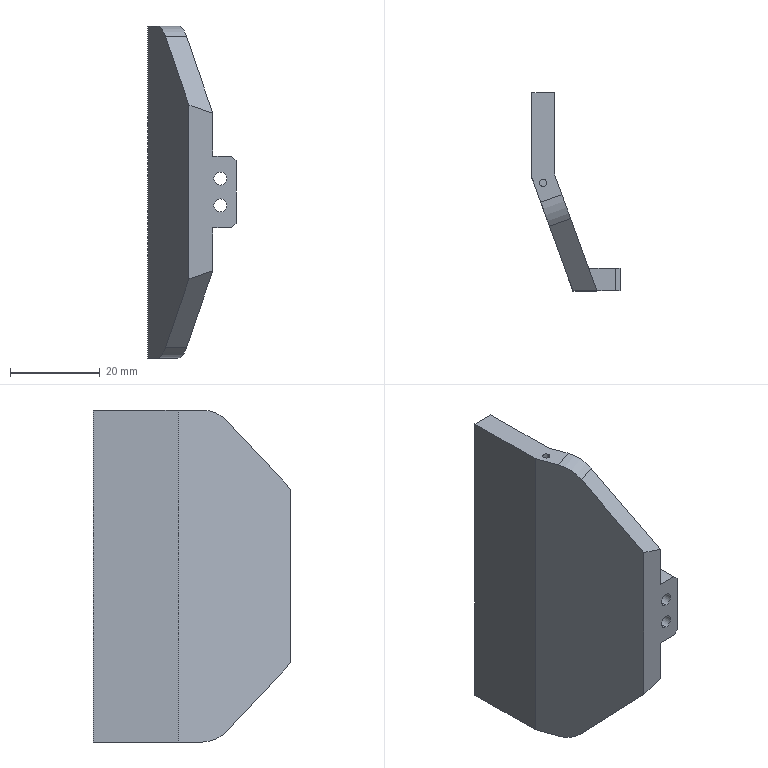NC program | NX | posted with a generic post | part box 19.643 x 44.061 x 74 mm
Lines 1 to 826 of 2613:
N10 G17 G21 G94 G90
(ADAPTIVE_MILLING , TOOL : D8开粗)
N12 T02 M6
N14 G54
N16 G17 G0 G90 X-47.558 Y-38.993 B0. C0. S6500 M3
N18 G43 Z30. H2
N20 Z-6.403
N22 G94 G1 X-47.492 Y-39.128 Z-7.34 F2500.
N24 X-47.426 Y-39.263 Z-7.711
N26 X-47.36 Y-39.398 Z-7.983
N28 X-47.294 Y-39.533 Z-8.203
N30 X-47.228 Y-39.667 Z-8.387
N32 X-47.163 Y-39.802 Z-8.546
N34 X-47.097 Y-39.937 Z-8.683
N36 X-47.031 Y-40.072 Z-8.803
N38 X-46.965 Y-40.207 Z-8.909
N40 X-46.899 Y-40.341 Z-9.001
N42 X-46.834 Y-40.476 Z-9.082
N44 X-46.768 Y-40.611 Z-9.153
N46 X-46.702 Y-40.746 Z-9.213
N48 X-46.636 Y-40.881 Z-9.265
N50 X-46.57 Y-41.015 Z-9.308
N52 X-46.505 Y-41.15 Z-9.343
N54 X-46.439 Y-41.285 Z-9.369
N56 X-46.373 Y-41.42 Z-9.388
N58 X-46.307 Y-41.554 Z-9.399
N60 X-46.241 Y-41.689 Z-9.403
N62 X-45.513 Y-43.182
N64 G3 X-43.999 Y-43.007 R0.808
N66 X-43.585 Y-39.981 R11.665
N68 X-43.499 Y-30.169 R281.498
N70 G1 X-43.498 Y-0.807
N72 G2 X-41.632 Y2.597 R4.521
N74 X-37.843 Y4.119 R8.422
N76 X-32.61 Y4.472 R35.063
N78 G1 X-24.735 Y4.499
N80 X38.215 Y4.497
N82 G2 X41.601 Y2.603 R4.555
N84 X43.114 Y-1.166 R8.498
N86 X43.471 Y-6.398 R34.669
N88 G1 X43.498 Y-14.273
N90 X43.499 Y-42.121
N92 G3 X43.654 Y-43.509 R4.062
N94 G1 X43.805 Y-43.722
N96 G3 X45.057 Y-43.547 R0.8
N98 X45.149 Y-42.984 Z-9.366 R0.86
N100 G1 X45.038 Y-41.99 Z-9.303
N102 G2 X46.322 Y-41.205 R0.804 F15000.
N104 G1 X46.546 Y-41.378
N106 X46.759 Y-41.564
N108 G2 X46.943 Y-41.919 R0.832
N110 X46.411 Y-42.865 Z-9.378 R0.816 F2500.
N112 G1 X46.05 Y-43.022 Z-9.403
N114 X44.62 Y-43.645
N116 G2 X43.577 Y-43.252 R0.8
N118 X43.283 Y-41.381 R6.234
N120 X43.199 Y-34.743 R157.881
N122 G1 X43.197 Y-11.856
N124 G3 X43.067 Y-3.796 R144.834
N126 X42.299 Y0.279 R13.658
N128 X39.053 Y3.396 R5.427
N130 X35.047 Y4.114 R12.873
N132 X26.723 Y4.198 R203.788
N134 G1 X-27.902 Y4.197
N136 G3 X-35.437 Y4.053 R122.134
N138 X-39.461 Y3.235 R12.737
N140 X-42.391 Y0.085 R5.405
N142 X-43.114 Y-3.92 R12.823
N144 X-43.199 Y-12.244 R201.638
N146 G1 Y-32.018
N148 G2 X-43.322 Y-40.262 R153.123
N150 X-43.694 Y-43.231 R28.567
N152 G1 X-43.797 Y-43.431
N154 G2 X-45.117 Y-43.393 R0.8
N156 G1 X-45.352 Y-43.028
N158 X-46.207 Y-41.697 Z-9.303
N160 G2 X-46.314 Y-40.913 R0.813 F15000.
N162 G1 X-46.22 Y-40.669
N164 X-46.111 Y-40.432
N166 G2 X-44.671 Y-41.106 R0.8
N168 G1 X-44.889 Y-41.749
N170 X-45.149 Y-42.535 Z-9.356 F2500.
N172 G3 X-44.987 Y-43.242 Z-9.403 R0.799
N174 X-43.655 Y-43.072 R0.8
N176 X-42.97 Y-40.45 R7.766
N178 X-42.712 Y-33.973 R62.177
N180 G1 X-42.699 Y-27.244
N182 X-42.698 Y-10.544
N184 G2 X-42.568 Y-3.91 R96.862
N186 X-41.825 Y-0.636 R9.476
N188 X-38.335 Y2.524 R6.635
N190 X-33.772 Y3.511 R14.696
N192 X-26.688 Y3.693 R98.536
N194 G1 X-21.252 Y3.713
N196 G3 X-20.829 Y3.886 R5.378
N198 G2 X-19.332 Y4.15 R4.834
N200 G1 X19.368
N202 G2 X21.088 Y3.911 R18.579
N204 G3 X26.996 Y3.706 R60.488
N206 G2 X34.526 Y3.606 R169.703
N208 X38.051 Y2.955 R11.35
N210 X41.428 Y-0.465 R6.487
N212 X42.494 Y-5.048 R13.967
N214 X42.694 Y-12.693 R97.602
N216 G1 X42.698 Y-17.156
N218 X42.7 Y-35.24
N220 G3 X42.822 Y-41.261 R87.83
N222 X43.278 Y-43.288 R5.747
N224 X43.917 Y-43.94 R1.116
N226 X44.864 Y-43.48 R0.8
N228 G1 X45.366 Y-41.98 Z-9.303
N230 X45.656 Y-41.11 F15000.
N232 X45.685 Y-40.985
N234 X45.697 Y-40.857
N236 Y-13.166
N238 G3 X45.047 Y-5.309 R47.833
N240 G1 X44.798 Y-3.797
N242 X44.532 Y-2.289
N244 G3 X43.545 Y0.807 R17.168
N246 X42.04 Y3.094 R7.735
N248 X40.398 Y4.429 R11.341
N250 X38.041 Y5.448 R8.159
N252 X35.622 Y5.838 R12.101
N254 G1 X22.704 Y6.583
N256 G3 X22.346 Y6.521 R0.848
N258 G1 X20.925 Y5.92
N260 X20.479 Y5.733 Z-9.334 F2500.
N262 X20.038 Y5.538 Z-9.364
N264 G3 X19.649 Y5.08 Z-9.403 R0.8
N266 X20.187 Y4.065 R0.8
N268 X22.184 Y3.527 R16.655
N270 X27.364 Y3.224 R38.873
N272 G2 X34.129 Y3.086 R136.962
N274 X37.786 Y2.097 R8.143
N276 X41.056 Y-1.974 R7.812
N278 X42.026 Y-7.039 R17.772
N280 X42.194 Y-14.911 R127.356
N282 G1 X42.198 Y-19.486
N284 X42.2 Y-34.378
N286 G3 X42.324 Y-40.628 R91.007
N288 X42.958 Y-43.254 R6.736
N290 X43.796 Y-43.971 R1.278
N292 G1 X43.871 Y-43.98
N294 G3 X44.579 Y-43.613 R0.801
N296 G1 X44.778 Y-43.303
N298 X45.632 Y-41.971 Z-9.303
N300 G2 X45.899 Y-41.635 R1.18 F15000.
N302 X46.388 Y-41.463 R0.808
N304 X46.821 Y-41.5 R1.214
N306 X47.296 Y-41.918 R0.804
N308 X46.786 Y-43.034 Z-9.391 R0.808 F2500.
N310 G1 X46.61 Y-43.098 Z-9.403
N312 X44.303 Y-43.931
N314 G2 X43.053 Y-43.523 R1.08
N316 X42.215 Y-41.341 R4.767
N318 X41.924 Y-36.863 R30.864
N320 G1 X41.898 Y-29.455
N322 X41.896 Y-16.293
N324 G3 X41.725 Y-7.371 R143.397
N326 X40.788 Y-2.452 R17.424
N328 X35.35 Y2.37 R7.418
N330 X30.735 Y2.861 R22.027
N332 G2 X24.11 Y3.051 R164.675
N334 X21.769 Y3.397 R10.417
N336 G1 X21.67 Y3.451
N338 G2 X21.32 Y4.104 R0.802
N340 X21.44 Y4.561 Z-9.373 R1.113
N342 G1 X21.858 Y5.584 Z-9.303
N344 X22.228 Y6.486 F15000.
N346 G2 X22.685 Y6.939 R0.865
N348 X23.09 Y5.434 R-0.8
N350 G1 X22.248 Y5.404
N352 X21.687 Y5.388 Z-9.339 F2500.
N354 X21.126 Y5.356 Z-9.374
N356 G3 X20.722 Y5.153 Z-9.403 R0.833
N358 X20.905 Y3.856 R0.8
N360 G2 X21.96 Y3.258 R7.341
N362 G3 X24.63 Y2.64 R8.31
N364 X30.643 Y2.357 R99.943
N366 G2 X34.91 Y1.801 R18.389
N368 X39.949 Y-2.699 R7.827
N370 X41.131 Y-7.641 R15.896
N372 X41.387 Y-14.984 R82.682
N374 G1 X41.398 Y-22.001
N376 G3 X41.449 Y-37.436 R879.459
N378 X41.892 Y-41.698 R20.187
N380 X42.926 Y-43.702 R4.096
N382 X43.88 Y-43.982 R1.117
N384 G2 X42.623 Y-43.495 R1.307
N386 X41.579 Y-41.16 R5.176
N388 X41.15 Y-36.518 R25.526
N390 G1 X41.145 Y-19.379
N392 G3 X41.008 Y-10.681 R945.326
N394 X40.341 Y-5.068 R27.166
N396 X38.029 Y-0.704 R9.4
N398 X33.507 Y1.619 R8.796
N400 X28.699 Y2.103 R29.519
N402 G2 X23.82 Y2.494 R39.677
N404 X22.323 Y2.934 R4.689
N406 G1 X21.781 Y3.362
N408 G3 X22.733 Y2.634 R9.351
N410 X25.412 Y1.917 R8.38
N412 X30.363 Y1.5 R118.082
N414 G2 X34.705 Y0.551 R14.276
N416 X39.219 Y-4.196 R8.509
N418 X40.35 Y-9.379 R17.768
N420 X40.602 Y-16.225 R107.207
N422 G1 X41.022 Y-18.03
N424 X41.145 Y-19.379
N426 X41.022 Y-18.03
N428 G2 X40.44 Y-15.438 R39.022
N430 X40.134 Y-10.68 R104.912
N432 G3 X39.213 Y-5.336 R21.349
N434 X35.445 Y-0.44 R8.814
N436 X30.799 Y1.059 R12.221
N438 X25.925 Y1.575 R367.233
N440 G2 X23.014 Y2.306 R9.794
N442 X22.399 Y2.854 R10.317
N444 G3 X23.483 Y1.953 R5.313
N446 X26.391 Y1.127 R9.502
N448 G2 X30.877 Y0.495 R147.307
N450 X35.39 Y-1.346 R10.613
N452 X38.687 Y-6.184 R9.709
N454 X39.616 Y-11.415 R22.702
N456 G3 X39.883 Y-14.49 R67.344
N458 G2 X40.576 Y-16.151 R17.83
N460 G3 X39.922 Y-14.595 R11.063
N462 G2 X39.513 Y-12.848 R6.153
N464 G3 X38.867 Y-8.288 R58.588
N466 X36.808 Y-3.465 R11.841
N468 X31.791 Y-0.177 R9.515
N470 X27.47 Y0.661 R32.558
N472 G2 X24.077 Y1.465 R15.345
N474 X23.626 Y1.702 R4.079
N476 G1 X23.052 Y2.241
N478 G3 X24.149 Y1.288 R7.408
N480 X26.87 Y0.366 R9.404
N482 G2 X30.968 Y-0.544 R55.8
N484 X36.359 Y-4.238 R9.731
N486 X38.359 Y-9.105 R13.149
N488 X39.064 Y-13.058 R287.789
N490 G1 X39.204 Y-13.357
N492 X39.877 Y-14.507
N494 G2 X39.003 Y-13.007 R36.74
N496 X38.298 Y-10.253 R18.539
N498 G3 X36.728 Y-5.653 R16.594
N500 X31.139 Y-1.064 R9.909
N502 X27.109 Y0.005 R38.547
N504 G2 X24.487 Y0.9 R10.548
N506 G1 X23.809 Y1.529
N508 G3 X24.971 Y0.506 R9.153
N510 X27.59 Y-0.523 R11.038
N512 G2 X31.561 Y-1.889 R25.851
N514 X36.764 Y-7.482 R10.349
N516 X38.015 Y-11.435 R34.206
N518 G3 X38.324 Y-12.218 R2.509
N520 G2 X39.146 Y-13.28 R13.068
N522 G3 X38.174 Y-12.024 R32.204
N524 G2 X37.226 Y-9.635 R14.568
N526 G3 X35.115 Y-5.375 R15.025
N528 X30.23 Y-1.785 R11.119
N530 X26.569 Y-0.495 R140.937
N532 G2 X25.366 Y0.066 R6.768
N534 G1 X24.656 Y0.733
N536 G3 X26.002 Y-0.45 R10.5
N538 X28.712 Y-1.703 R18.552
N540 G2 X32.897 Y-4.094 R14.898
N542 X36.11 Y-8.558 R12.561
N544 G3 X37.205 Y-11.036 R113.313
N546 G1 X38.279 Y-12.17
N548 G3 X37.121 Y-10.959 R64.393
N550 G2 X35.838 Y-8.65 R19.314
N552 G3 X32.076 Y-4.004 R13.088
N554 X28.378 Y-1.939 R19.144
N556 G2 X26.504 Y-1.003 R18.276
N558 G1 X25.602 Y-0.156
N560 G3 X27.185 Y-1.594 R19.225
N562 X29.968 Y-3.274 R61.086
N564 G2 X35.017 Y-8.465 R14.517
N566 G3 X35.809 Y-9.747 R59.821
N568 G1 X37.226 Y-11.081
N570 G2 X35.436 Y-9.355 R32.559
N572 G3 X33.354 Y-6.667 R93.163
N574 X29.044 Y-3.131 R17.686
N576 G1 X28.186 Y-2.584
N578 X26.874 Y-1.351
N580 G3 X31.179 Y-5.27 R103.859
N582 G2 X32.686 Y-6.813 R33.054
N584 G1 X35.692 Y-9.637
N586 X29.325 Y-3.654
N588 G2 X29.997 Y-2.281 R0.8
N590 G1 X30.216 Y-2.348 Z-9.389
N592 X30.422 Y-2.447 Z-9.374
N594 X31.434 Y-2.934 Z-9.303
N596 X32.811 Y-3.602 F15000.
N598 X33.932 Y-4.489
N600 X35.039 Y-5.392
N602 G2 X37.325 Y-7.571 R27.569
N604 G1 X39.688 Y-10.1
N606 G2 X41.974 Y-13.298 R14.846
N608 X43.341 Y-17.981 R12.301
N610 X43.562 Y-22.418 R55.793
N612 G1 X43.667 Y-34.001
N614 G2 X43.305 Y-34.678 R0.801
N616 G1 X43.142 Y-34.784
N618 X41.817 Y-35.65 Z-9.403 F2500.
N620 X41.609 Y-35.784
N622 X41.408 Y-35.929
N624 G3 X41.15 Y-36.518 R0.803
N626 X41.169 Y-40.457 R119.323
N628 X42.245 Y-43.427 R5.4
N630 X43.16 Y-43.996 R1.328
N632 G1 X43.535 Y-43.989
N634 G2 X42.724 Y-43.903 R1.567
N636 X41.464 Y-42.367 R3.059
N638 X41.15 Y-41.365 R5.067
N640 G1 Y-40.128
N642 G3 X41.184 Y-42.001 R15.776
N644 X42.446 Y-43.934 R2.778
N646 X43.096 Y-43.998 R1.442
N648 G2 X41.814 Y-43.517 R1.365
N650 X41.15 Y-42.276 R2.436
N652 G1 Y-41.676
N654 G3 X41.203 Y-42.761 R4.162
N656 X42.176 Y-43.969 R1.81
N658 X42.712 Y-44.006 R1.858
N660 G2 X41.421 Y-43.407 R1.262
N662 X41.15 Y-42.432 R1.267
N664 G3 X41.409 Y-43.575 R1.678
N666 X42.408 Y-44.012 R0.977
N668 G2 X41.15 Y-42.89 R1.063
N670 G3 X41.587 Y-43.91 R1.019
N672 X42.111 Y-44.018 R1.051
N674 G2 X41.162 Y-43.3 R0.843
N676 X41.685 Y-42.456 R0.808
N678 G1 X43.128 Y-41.92
N680 X43.268 Y-41.868 Z-9.399
N682 X43.409 Y-41.816 Z-9.388
N684 X43.549 Y-41.764 Z-9.369
N686 X43.69 Y-41.711 Z-9.343
N688 X43.831 Y-41.659 Z-9.308
N690 X43.971 Y-41.607 Z-9.265
N692 X44.112 Y-41.555 Z-9.213
N694 X44.253 Y-41.503 Z-9.153
N696 X44.393 Y-41.45 Z-9.082
N698 X44.534 Y-41.398 Z-9.001
N700 X44.674 Y-41.346 Z-8.909
N702 X44.815 Y-41.294 Z-8.803
N704 X44.956 Y-41.242 Z-8.683
N706 X45.096 Y-41.19 Z-8.546
N708 X45.237 Y-41.137 Z-8.387
N710 X45.378 Y-41.085 Z-8.203
N712 X45.518 Y-41.033 Z-7.983
N714 X45.659 Y-40.981 Z-7.711
N716 X45.799 Y-40.929 Z-7.34
N718 X45.94 Y-40.876 Z-6.403
N720 G0 Z30.
N722 X-49.529 Y-41.484
N724 Z-6.403
N726 G1 X-49.379 Y-41.493 Z-7.34
N728 X-49.23 Y-41.503 Z-7.711
N730 X-49.08 Y-41.512 Z-7.983
N732 X-48.93 Y-41.521 Z-8.203
N734 X-48.78 Y-41.531 Z-8.387
N736 X-48.631 Y-41.54 Z-8.546
N738 X-48.481 Y-41.549 Z-8.683
N740 X-48.331 Y-41.559 Z-8.803
N742 X-48.182 Y-41.568 Z-8.909
N744 X-48.032 Y-41.577 Z-9.001
N746 X-47.882 Y-41.587 Z-9.082
N748 X-47.732 Y-41.596 Z-9.153
N750 X-47.583 Y-41.605 Z-9.213
N752 X-47.433 Y-41.615 Z-9.265
N754 X-47.283 Y-41.624 Z-9.308
N756 X-47.134 Y-41.634 Z-9.343
N758 X-46.984 Y-41.643 Z-9.369
N760 X-46.834 Y-41.652 Z-9.388
N762 X-46.685 Y-41.662 Z-9.399
N764 X-46.535 Y-41.671 Z-9.403
N766 G2 X-45.891 Y-42.064 R0.81
N768 G1 X-45.121 Y-43.357
N770 G3 X-43.85 Y-43.509 R0.808
N772 X-42.874 Y-41.628 R4.068
N774 X-42.316 Y-37.312 R20.428
N776 X-42.2 Y-27.318 R253.742
N778 G1 X-42.199 Y-14.582
N780 G2 X-42.123 Y-5.445 R250.902
N782 X-41.535 Y-2.1 R10.375
N784 X-37.642 Y1.803 R7.325
N786 X-32.96 Y2.941 R14.861
N788 X-25.954 Y3.188 R78.231
N790 G3 X-22.128 Y3.24 R61.219
N792 X-21.517 Y3.554 R1.231
N794 G1 X-21.078 Y3.766
N796 G3 X-21.86 Y3.304 R2.911
N798 G2 X-23.435 Y3.004 R4.68
N800 X-29.531 Y2.831 R185.373
N802 G3 X-35.005 Y2.257 R28.775
N804 X-39.179 Y0.222 R9.177
N806 X-41.442 Y-3.948 R7.683
N808 X-41.862 Y-8.496 R24.344
N810 X-41.899 Y-14.683 R583.034
N812 G1 X-41.901 Y-28.117
N814 G2 X-42.052 Y-37.652 R183.218
N816 X-42.703 Y-41.809 R17.143
N818 X-43.668 Y-43.594 R5.171
N820 G1 X-43.822 Y-43.699
N822 G2 X-44.912 Y-43.303 R0.8
N824 X-44.896 Y-42.622 Z-9.359 R0.839
N826 G1 X-44.574 Y-41.802 Z-9.303
N828 G3 X-44.45 Y-41.359 R1.283 F15000.
N830 X-45.628 Y-40.629 R0.801
N832 X-45.999 Y-41.689 R0.8
N834 G1 X-45.868 Y-41.891 Z-9.318 F2500.
N836 X-45.721 Y-42.082 Z-9.334
N838 X-45.054 Y-42.956 Z-9.403
N840 X-44.836 Y-43.246
N842 X-44.605 Y-43.526
N844 G3 X-43.848 Y-43.712 R0.801
N846 X-43.09 Y-43.075 R1.579
N848 X-41.997 Y-40.371 R6.959
N850 X-41.476 Y-34.829 R32.124
N852 X-41.4 Y-23.794 R510.12
N854 G2 X-41.351 Y-8.67 R843.284
N856 X-40.825 Y-4.174 R19.337
N858 X-36.301 Y0.952 R7.816
N860 X-31.287 Y2.14 R16.018
N862 X-25.006 Y2.438 R115.742
N864 G3 X-22.601 Y2.737 R10.648
N866 X-22.133 Y3.102 R1.749
N868 G1 X-21.8 Y3.346
N870 G3 X-22.46 Y2.796 R5.528
N872 G2 X-24.127 Y2.31 R4.219
N874 X-29.038 Y1.99 R69.166
N876 G3 X-34.407 Y1.214 R23.913
N878 X-38.837 Y-1.562 R8.757
N880 X-40.713 Y-6.003 R9.47
N882 X-41.078 Y-11.46 R35.54
N884 G1 X-41.1 Y-18.834
N886 X-41.15 Y-19.555
N888 X-41.157 Y-33.641
N890 G2 X-41.613 Y-39.696 R39.833
N892 X-42.691 Y-42.791 R8.55
N894 X-43.749 Y-43.774 R2.351
N896 G1 X-43.971 Y-43.811
N898 G2 X-44.756 Y-43.342 R0.881
N900 X-44.826 Y-42.684 Z-9.36 R0.926
N902 G1 X-44.649 Y-41.797 Z-9.303
N904 X-43.129 Y-34.202 F15000.
N906 X-42.876 Y-32.959 Z-9.383 F2500.
N908 X-42.822 Y-32.812 Z-9.393
N910 X-42.744 Y-32.677 Z-9.403
N912 G2 X-41.15 Y-33.192 R0.88
N914 X-41.177 Y-38.09 R126.917
N916 X-42.174 Y-42.257 R11.263
N918 X-43.485 Y-43.753 R3.254
N920 G1 X-43.813 Y-43.822
N922 G2 X-44.529 Y-43.327 R0.801
N924 X-44.506 Y-42.659 Z-9.36 R0.841
N926 G1 X-44.177 Y-41.827 Z-9.303
N928 X-44.081 Y-41.589 F15000.
N930 X-43.999 Y-41.344
N932 G3 X-44.735 Y-40.383 R0.8
N934 X-45.212 Y-40.398 R1.417
N936 X-45.699 Y-41.556 R0.8
N938 G1 X-45.617 Y-41.705
N940 X-44.851 Y-43.09 Z-9.403 F2500.
N942 X-44.735 Y-43.303
N944 X-44.606 Y-43.509
N946 G3 X-44.03 Y-43.809 R0.803
N948 X-42.763 Y-43.386 R1.405
N950 X-41.326 Y-40.922 R5.527
N952 G1 X-41.15 Y-40.251
N954 Y-37.476
N956 G2 X-41.173 Y-40.657 R57.979
N958 X-42.764 Y-43.553 R4.543
N960 X-43.704 Y-43.83 R1.169
N962 G3 X-42.268 Y-43.336 R1.645
N964 X-41.153 Y-41.564 R3.596
N966 G1 X-41.15 Y-40.364
N968 G2 X-41.17 Y-41.767 R18.293
N970 X-42.877 Y-43.836 R2.913
N972 X-43.365 Y-43.851 R1.911
N974 G3 X-41.817 Y-43.307 R1.722
N976 X-41.154 Y-42.256 R2.022
N978 G1 X-41.15 Y-41.577
N980 G2 X-41.176 Y-42.453 R5.021
N982 X-42.608 Y-43.882 R2.091
N984 G1 X-42.99 Y-43.874
N986 G3 X-41.375 Y-43.187 R1.624
N988 X-41.15 Y-42.278 R1.221
N990 G2 X-41.295 Y-43.156 R1.491
N992 X-42.399 Y-43.911 R1.431
N994 G1 X-42.586 Y-43.899
N996 G3 X-41.157 Y-43.016 R1.202
N998 G1 X-41.15 Y-42.679
N1000 G2 X-42.126 Y-43.928 R1.078
N1002 G1 X-42.314 Y-43.916
N1004 G3 X-41.211 Y-43.393 R0.968
N1006 X-41.15 Y-42.954 R1.67
N1008 G2 X-41.871 Y-43.923 R0.858
N1010 X-42.718 Y-43.372 R0.801
N1012 G1 X-43.247 Y-41.881 Z-9.303
N1014 X-43.408 Y-41.409 F15000.
N1016 X-43.428 Y-41.225
N1018 X-43.302 Y-21.037
N1020 G2 X-43.133 Y-20.55 R0.808
N1022 X-42.8 Y-20.284 Z-9.33 R1.152 F2500.
N1024 G1 X-41.825 Y-19.668 Z-9.403
N1026 X-41.595 Y-19.524
N1028 X-41.371 Y-19.369
N1030 G3 X-41.1 Y-18.834 R0.805
N1032 G2 X-40.821 Y-16.948 R14.712
N1034 G3 X-40.588 Y-11.76 R56.833
N1036 G2 X-40.204 Y-6.567 R33.849
N1038 X-37.862 Y-1.782 R8.818
N1040 X-33.153 Y0.773 R10.149
N1042 X-28.149 Y1.489 R27.421
N1044 G3 X-24.085 Y1.892 R36.02
N1046 X-23.043 Y2.247 R2.545
N1048 G1 X-22.414 Y2.838
N1050 G2 X-23.228 Y2.101 R13.386
N1052 X-25.446 Y1.483 R6.483
N1054 X-30.17 Y0.983 R736.72
N1056 G3 X-35.034 Y-0.348 R15.306
N1058 X-39.563 Y-5.923 R8.617
N1060 X-40.232 Y-10.891 R21.716
N1062 G2 X-40.444 Y-15.747 R123.576
N1064 G3 X-40.846 Y-17.129 R79.581
N1066 G2 X-40.227 Y-15.14 R30.828
N1068 G3 X-39.826 Y-11.949 R19.988
N1070 G2 X-39.245 Y-7.192 R29.966
N1072 X-33.568 Y-0.581 R9.033
N1074 X-28.762 Y0.559 R19.744
N1076 G3 X-24.811 Y1.157 R41.772
N1078 X-23.809 Y1.528 R2.771
N1080 G1 X-23.071 Y2.221
N1082 G2 X-23.992 Y1.38 R31.386
N1084 X-26.312 Y0.654 R7.204
N1086 G3 X-30.747 Y-0.109 R106.458
N1088 X-35.435 Y-2.117 R12.108
N1090 X-38.807 Y-7.344 R9.383
N1092 X-39.451 Y-11.376 R24.767
N1094 G2 X-39.849 Y-14.471 R26.037
N1096 G3 X-40.339 Y-15.506 R25.232
N1098 G2 X-39.636 Y-14.057 R25.835
N1100 G3 X-39.058 Y-11.558 R12.835
N1102 G2 X-38.166 Y-7.349 R25.483
N1104 X-32.536 Y-1.421 R9.525
N1106 X-28.314 Y-0.248 R21.997
N1108 G3 X-24.908 Y0.58 R21.749
N1110 G1 X-24.665 Y0.723
N1112 X-23.845 Y1.494
N1114 G2 X-24.854 Y0.57 R35.832
N1116 X-27.173 Y-0.258 R8.294
N1118 G3 X-31.38 Y-1.376 R40.038
N1120 X-36.252 Y-4.766 R10.257
N1122 X-38.279 Y-9.368 R12.001
N1124 G2 X-39.069 Y-13.042 R143.624
N1126 X-39.416 Y-13.685 R1.583
N1128 G1 X-39.719 Y-14.245
N1130 G2 X-38.95 Y-12.997 R11.775
N1132 G3 X-38.185 Y-10.821 R11.785
N1134 G2 X-36.704 Y-6.776 R18.716
N1136 X-31.481 Y-2.189 R10.392
N1138 X-27.248 Y-0.811 R36.397
N1140 G3 X-25.693 Y-0.236 R7.987
N1142 G1 X-24.742 Y0.65
N1144 G2 X-25.94 Y-0.423 R10.47
N1146 X-28.433 Y-1.424 R13.096
N1148 G3 X-32.689 Y-3.246 R19.463
N1150 X-37.091 Y-8.695 R10.778
N1152 X-38.244 Y-11.978 R340.285
N1154 G2 X-38.62 Y-12.558 R1.404
N1156 G1 X-39.053 Y-13.17
N1158 G2 X-38.137 Y-11.993 R13.181
N1160 G3 X-36.987 Y-9.665 R16.332
N1162 G2 X-34.28 Y-5.46 R13.464
N1164 X-29.801 Y-2.582 R13.632
N1166 G3 X-26.914 Y-1.376 R59.363
N1168 G1 X-25.72 Y-0.268
N1170 G2 X-27.123 Y-1.55 R21.102
N1172 X-29.694 Y-2.852 R21.937
N1174 G3 X-34.121 Y-5.924 R14.02
N1176 X-36.678 Y-9.853 R15.94
N1178 G2 X-37.463 Y-11.31 R10.806
N1180 G1 X-38.274 Y-12.174
N1182 G2 X-36.993 Y-10.821 R76.533
N1184 G3 X-35.232 Y-8.259 R69.939
N1186 G2 X-29.928 Y-3.664 R14.942
N1188 G1 X-28.475 Y-2.857
N1190 X-26.917 Y-1.393
N1192 G2 X-28.931 Y-3.245 R39.434
N1194 G3 X-31.891 Y-5.318 R81.276
N1196 X-34.728 Y-7.929 R37.129
N1198 G2 X-36.087 Y-10.008 R67.586
N1200 G1 X-37.199 Y-11.054
N1202 G3 X-33.52 Y-7.49 R150.399
N1204 G2 X-31.849 Y-6.027 R40.984
N1206 G1 X-28.624 Y-2.997
N1208 X-35.511 Y-9.468
N1210 G2 X-36.736 Y-9.329 R0.808
N1212 G1 X-37.317 Y-8.463
N1214 X-37.401 Y-8.338 Z-9.399
N1216 X-37.485 Y-8.214 Z-9.388
N1218 X-37.568 Y-8.089 Z-9.369
N1220 X-37.652 Y-7.964 Z-9.343
N1222 X-37.735 Y-7.84 Z-9.308
N1224 X-37.819 Y-7.715 Z-9.265
N1226 X-37.903 Y-7.591 Z-9.213
N1228 X-37.986 Y-7.466 Z-9.153
N1230 X-38.07 Y-7.342 Z-9.082
N1232 X-38.153 Y-7.217 Z-9.001
N1234 X-38.237 Y-7.093 Z-8.909
N1236 X-38.321 Y-6.968 Z-8.803
N1238 X-38.404 Y-6.844 Z-8.683
N1240 X-38.488 Y-6.719 Z-8.546
N1242 X-38.572 Y-6.595 Z-8.387
N1244 X-38.655 Y-6.47 Z-8.203
N1246 X-38.739 Y-6.346 Z-7.983
N1248 X-38.822 Y-6.221 Z-7.711
N1250 X-38.906 Y-6.096 Z-7.34
N1252 X-38.99 Y-5.972 Z-6.403
N1254 G0 Z30.
N1256 X-28.209 Y4.157
N1258 Z-5.472
N1260 G1 X-28.088 Y4.068 Z-6.408
N1262 X-27.968 Y3.979 Z-6.779
N1264 X-27.847 Y3.89 Z-7.052
N1266 X-27.726 Y3.801 Z-7.272
N1268 X-27.605 Y3.712 Z-7.456
N1270 X-27.485 Y3.623 Z-7.614
N1272 X-27.364 Y3.534 Z-7.751
N1274 X-27.243 Y3.445 Z-7.872
N1276 X-27.122 Y3.356 Z-7.977
N1278 X-27.001 Y3.267 Z-8.07
N1280 X-26.881 Y3.178 Z-8.151
N1282 X-26.76 Y3.089 Z-8.221
N1284 X-26.639 Y3. Z-8.282
N1286 X-26.518 Y2.911 Z-8.333
N1288 X-26.398 Y2.822 Z-8.376
N1290 X-26.277 Y2.733 Z-8.411
N1292 X-26.156 Y2.645 Z-8.438
N1294 X-26.035 Y2.556 Z-8.457
N1296 X-25.915 Y2.467 Z-8.468
N1298 X-25.794 Y2.378 Z-8.472
N1300 X-24.677 Y1.555
N1302 G3 X-23.699 Y1.57 R0.808
N1304 G2 X-19.804 Y3.211 R8.624
N1306 X-14.911 Y3.587 R31.074
N1308 X-6.737 Y3.63 R646.155
N1310 G1 X17.63 Y3.647
N1312 G2 X21.116 Y2.598 R7.579
N1314 G3 X21.724 Y2.502 R6.
N1316 G2 X23.76 Y1.521 R4.933
N1318 G3 X21.155 Y2.569 R4.663
N1320 X16.069 Y3.301 R18.041
N1322 X10.819 Y3.342 R557.9
N1324 G1 X-17.211 Y3.34
N1326 G3 X-20.767 Y2.599 R26.726
N1328 X-23.195 Y1.911 R4.99
N1330 G2 X-20.804 Y2.597 R4.92
N1332 G3 X-17.958 Y2.736 R30.841
N1334 G2 X-9.934 Y2.84 R190.326
N1336 G1 X16.727 Y2.841
N1338 X18.472 Y2.597
N1340 X20.926
N1342 X21.224 Y2.561
N1344 X20.926 Y2.597
N1346 X-19.965
N1348 G2 X-20.765 Y3.289 R0.808
N1350 G1 X-20.951 Y4.573
N1352 X-20.972 Y4.721 Z-8.468
N1354 X-20.994 Y4.87 Z-8.457
N1356 X-21.015 Y5.018 Z-8.438
N1358 X-21.037 Y5.167 Z-8.411
N1360 X-21.058 Y5.315 Z-8.376
N1362 X-21.08 Y5.464 Z-8.333
N1364 X-21.101 Y5.612 Z-8.282
N1366 X-21.122 Y5.76 Z-8.221
N1368 X-21.144 Y5.909 Z-8.151
N1370 X-21.165 Y6.057 Z-8.07
N1372 X-21.187 Y6.206 Z-7.977
N1374 X-21.208 Y6.354 Z-7.872
N1376 X-21.23 Y6.503 Z-7.751
N1378 X-21.251 Y6.651 Z-7.614
N1380 X-21.273 Y6.8 Z-7.456
N1382 X-21.294 Y6.948 Z-7.272
N1384 X-21.316 Y7.097 Z-7.052
N1386 X-21.337 Y7.245 Z-6.779
N1388 X-21.359 Y7.393 Z-6.408
N1390 X-21.38 Y7.542 Z-5.472
N1392 G0 Z30.
N1394 X-31.003 Y1.527
N1396 Z-4.54
N1398 G1 X-30.882 Y1.439 Z-5.477
N1400 X-30.76 Y1.351 Z-5.848
N1402 X-30.639 Y1.262 Z-6.12
N1404 X-30.518 Y1.174 Z-6.34
N1406 X-30.397 Y1.086 Z-6.524
N1408 X-30.275 Y0.997 Z-6.682
N1410 X-30.154 Y0.909 Z-6.82
N1412 X-30.033 Y0.821 Z-6.94
N1414 X-29.912 Y0.733 Z-7.046
N1416 X-29.79 Y0.644 Z-7.138
N1418 X-29.669 Y0.556 Z-7.219
N1420 X-29.548 Y0.468 Z-7.29
N1422 X-29.427 Y0.379 Z-7.35
N1424 X-29.305 Y0.291 Z-7.402
N1426 X-29.184 Y0.203 Z-7.445
N1428 X-29.063 Y0.114 Z-7.479
N1430 X-28.942 Y0.026 Z-7.506
N1432 X-28.82 Y-0.062 Z-7.525
N1434 X-28.699 Y-0.15 Z-7.536
N1436 X-28.578 Y-0.239 Z-7.54
N1438 X-27.454 Y-1.057
N1440 G3 X-26.477 Y-1.038 R0.808
N1442 G2 X-25.551 Y-0.431 R7.215
N1444 X-23.665 Y0.843 R16.172
N1446 X-19.623 Y1.888 R11.292
N1448 X-12.728 Y2.092 R79.005
N1450 G1 X-7.741 Y2.096
N1452 X19.134 Y2.094
N1454 G2 X23.225 Y0.773 R7.9
N1456 G1 X24.469 Y-0.068
N1458 G2 X26.175 Y-0.799 R6.417
N1460 G1 X26.469 Y-1.032
N1462 G3 X25.387 Y-0.374 R5.127
N1464 G2 X22.908 Y0.651 R12.837
N1466 G3 X18.556 Y1.684 R11.373
N1468 X12.446 Y1.795 R108.209
N1470 G1 X-8.879 Y1.796
N1472 G3 X-18.065 Y1.68 R190.008
N1474 X-22.259 Y0.939 R14.434
N1476 X-24.287 Y-0.044 R21.874
N1478 X-25.879 Y-0.64 R4.987
N1480 G2 X-23.987 Y-0.006 R4.826
N1482 X-19.075 Y1.008 R30.676
N1484 X-11.958 Y1.283 R73.893
N1486 G1 X-4.908 Y1.296
N1488 X19.687 Y1.294
N1490 G2 X21.876 Y0.484 R14.753
N1492 G3 X23.006 Y0.041 R6.718
N1494 G2 X24.536 Y-0.092 R6.063
N1496 G3 X22.937 Y0.037 R5.965
N1498 G2 X21.061 Y0.528 R18.188
N1500 G3 X16.779 Y0.96 R20.312
N1502 X9.429 Y0.996 R616.269
N1504 G1 X-19.501
N1506 X-19.633 Y1.006
N1508 X-19.76 Y1.039
N1510 X-19.881 Y1.091
N1512 G2 X-20.303 Y1.738 Z-7.489 R0.832
N1514 G1 X-20.433 Y2.505 Z-7.44
N1516 X-20.555 Y3.218 F15000.
N1518 G3 X-22.019 Y3.513 R0.8
N1520 G1 X-22.192 Y3.236
N1522 X-22.376 Y2.966
N1524 X-22.456 Y2.887
N1526 X-22.544 Y2.817
N1528 X-23.761 Y2.015
N1530 X-24.696 Y1.392 Z-7.511 F2500.
N1532 G3 X-24.96 Y1.026 Z-7.54 R0.805
N1534 X-24.089 Y-0.027 R0.8
N1536 G2 X-22.86 Y0.056 R8.856
N1538 X-15.228 Y0.483 R55.047
N1540 G1 X-8.328 Y0.495
N1542 X18.974 Y0.493
N1544 X20.89 Y0.037
N1546 X22.99
N1548 G2 X18.704 Y0.146 R51.381
N1550 G3 X11.129 Y0.195 R458.888
N1552 G1 X-19.164 Y0.193
N1554 X-20.435 Y0.037
N1556 X-23.172
N1558 X20.703
N1560 G3 X21.505 Y0.942 R0.808
N1562 G1 X21.376 Y2.015
N1564 X21.358 Y2.164 Z-7.536
N1566 X21.34 Y2.313 Z-7.525
N1568 X21.322 Y2.462 Z-7.506
N1570 X21.304 Y2.611 Z-7.479
N1572 X21.286 Y2.76 Z-7.445
N1574 X21.268 Y2.909 Z-7.402
N1576 X21.251 Y3.058 Z-7.35
N1578 X21.233 Y3.206 Z-7.29
N1580 X21.215 Y3.355 Z-7.219
N1582 X21.197 Y3.504 Z-7.138
N1584 X21.179 Y3.653 Z-7.046
N1586 X21.161 Y3.802 Z-6.94
N1588 X21.143 Y3.951 Z-6.82
N1590 X21.125 Y4.1 Z-6.682
N1592 X21.107 Y4.249 Z-6.524
N1594 X21.089 Y4.398 Z-6.34
N1596 X21.072 Y4.547 Z-6.12
N1598 X21.054 Y4.696 Z-5.848
N1600 X21.036 Y4.845 Z-5.477
N1602 X21.018 Y4.994 Z-4.54
N1604 G0 Z30.
N1606 X-33.714 Y-1.052
N1608 Z-3.608
N1610 G1 X-33.591 Y-1.139 Z-4.545
N1612 X-33.469 Y-1.225 Z-4.916
N1614 X-33.347 Y-1.312 Z-5.189
N1616 X-33.224 Y-1.399 Z-5.408
N1618 X-33.102 Y-1.485 Z-5.593
N1620 X-32.979 Y-1.572 Z-5.751
N1622 X-32.857 Y-1.659 Z-5.888
N1624 X-32.734 Y-1.745 Z-6.008
N1626 X-32.612 Y-1.832 Z-6.114
N1628 X-32.489 Y-1.918 Z-6.207
N1630 X-32.367 Y-2.005 Z-6.288
N1632 X-32.244 Y-2.092 Z-6.358
N1634 X-32.122 Y-2.178 Z-6.419
N1636 X-32. Y-2.265 Z-6.47
N1638 X-31.877 Y-2.352 Z-6.513
N1640 X-31.755 Y-2.438 Z-6.548
N1642 X-31.632 Y-2.525 Z-6.575
N1644 X-31.51 Y-2.611 Z-6.593
N1646 X-31.387 Y-2.698 Z-6.605
N1648 X-31.265 Y-2.785 Z-6.608
N1650 X-30.126 Y-3.59